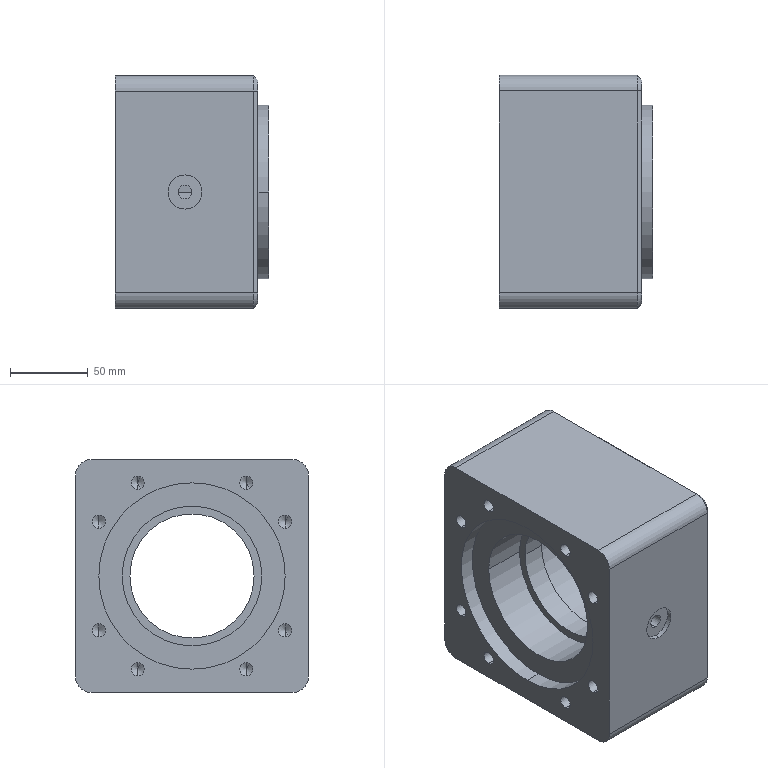Part | SolidWorks | features ICE 13, HoleWzd 4, Chamfer 2, CirPattern 1, Extrusion 1, Fillet 1 | 1 solid | 101 faces | box 99 x 150 x 150 mm | volume 1431839 mm3 | cylinder 50 | cone 36 | plane 15 | commonest cylinder face diameters 8.5 x16 3.3 x8 14 x8 20 x4 90 x4 8.8 x2